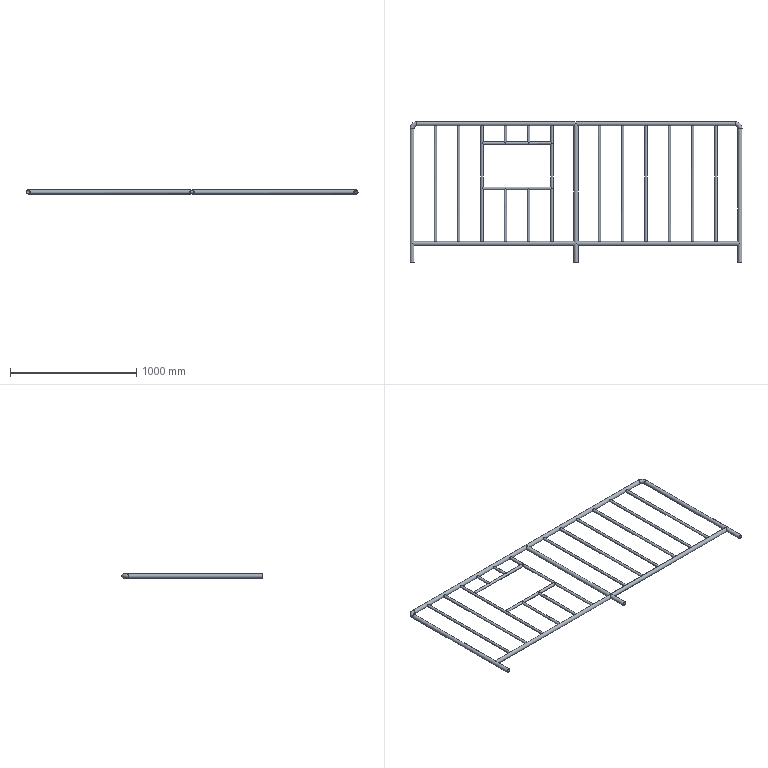Part | STEP file | PN_0055 304 guardrail 2600X1100_Default<As Machined> | 24 solids | 96 faces | box 2632 x 1116 x 32 mm | volume 2872572 mm3 | cylinder 81 | plane 11 | torus 4 | commonest cylinder face diameters 32 x35 20 x24 16 x16 28 x6